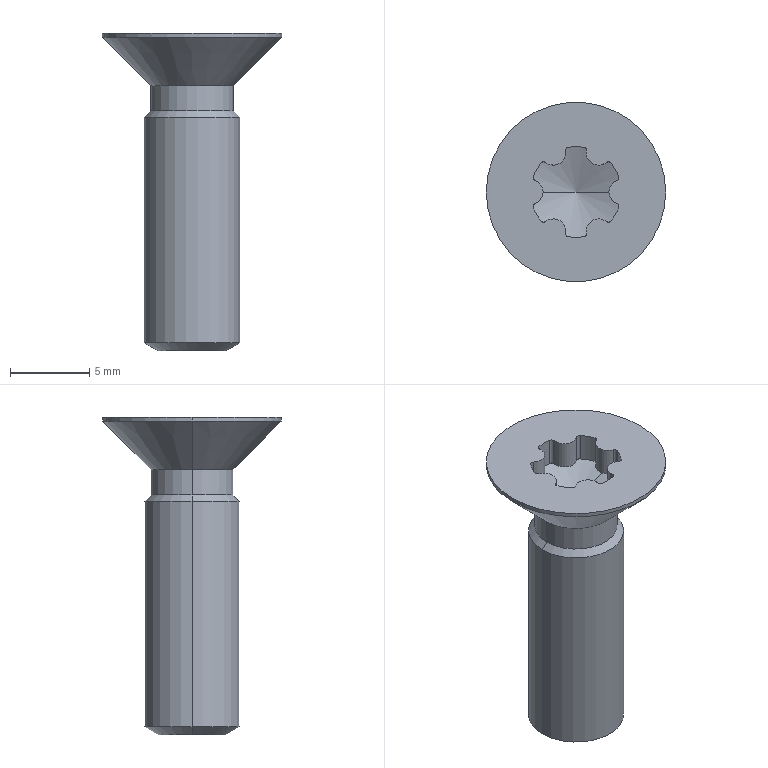Part | STEP file | 1 solid | 53 faces | box 11.3 x 11.3 x 20 mm | volume 605.952 mm3 | cylinder 37 | plane 8 | cone 8 | commonest cylinder face diameters 0.4 x16 1.57 x9 5.72 x6 5.196 x2 6 x2 11.3 x2